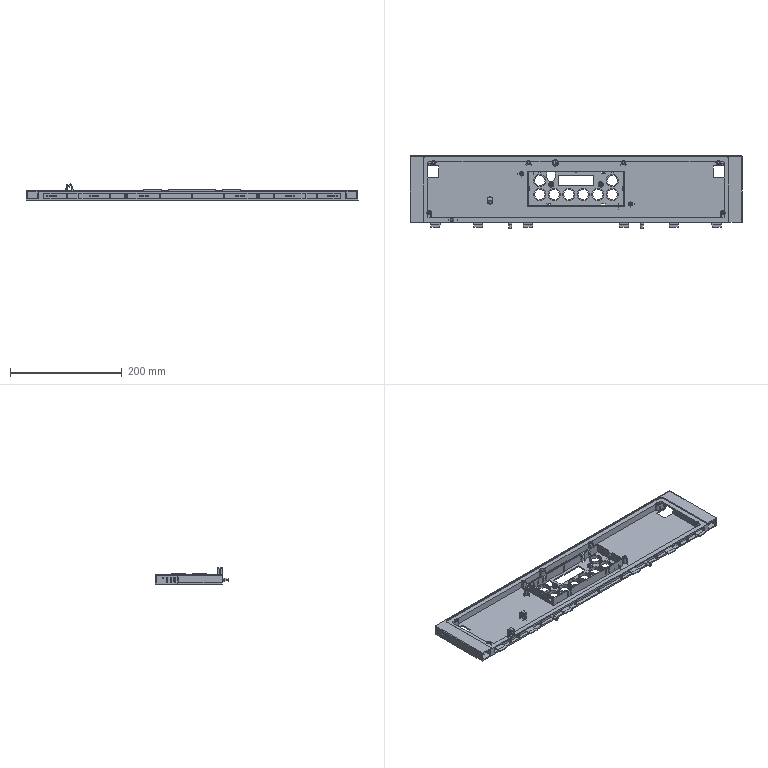Part | STEP file | ZXW722-L-27 | 1 solid | 766 faces | box 595 x 131 x 28.9 mm | volume 264991 mm3 | plane 552 | cylinder 192 | cone 10 | torus 10 | spline 2 | commonest cylinder face diameters 1 x46 2 x24 8.5 x18 19 x16 22 x16 3.2 x12